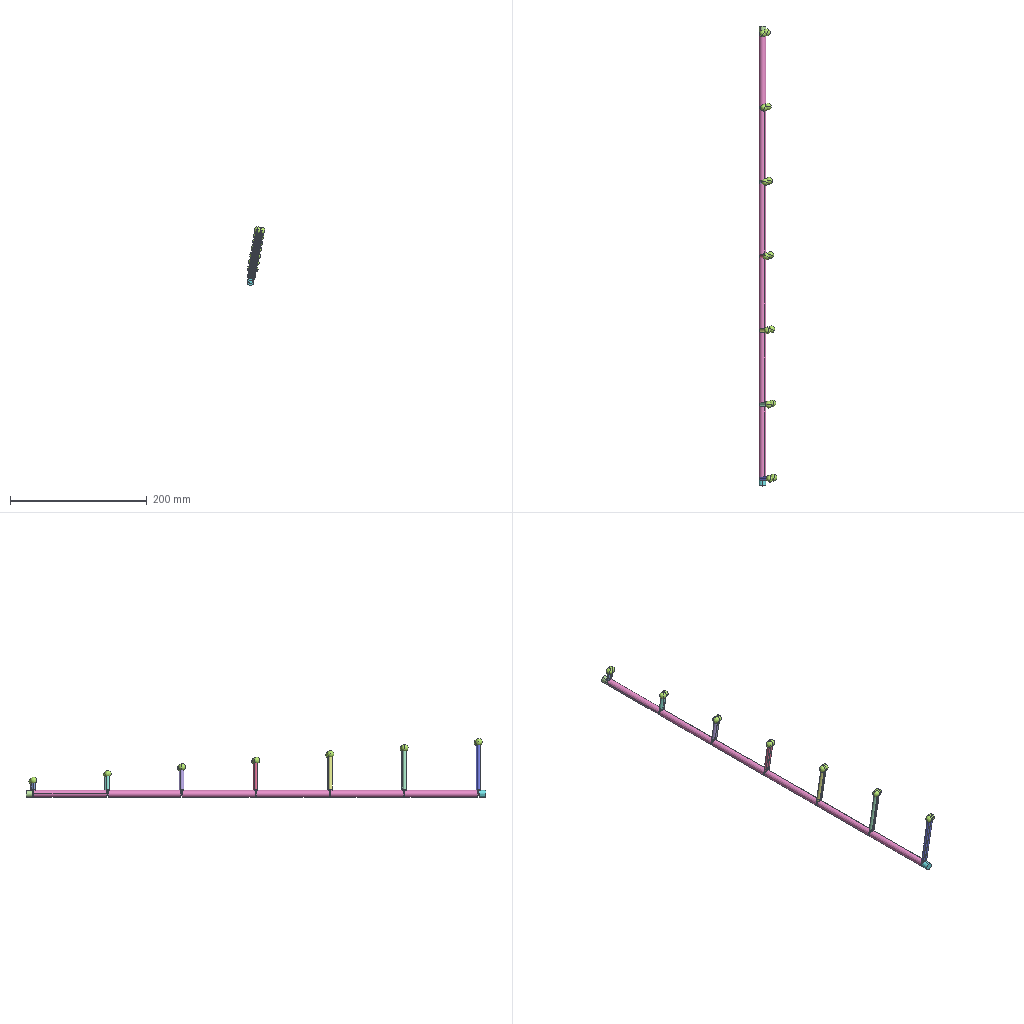Assembly | SolidWorks | 18 different items | 43 placed | box 26 x 673 x 86 mm
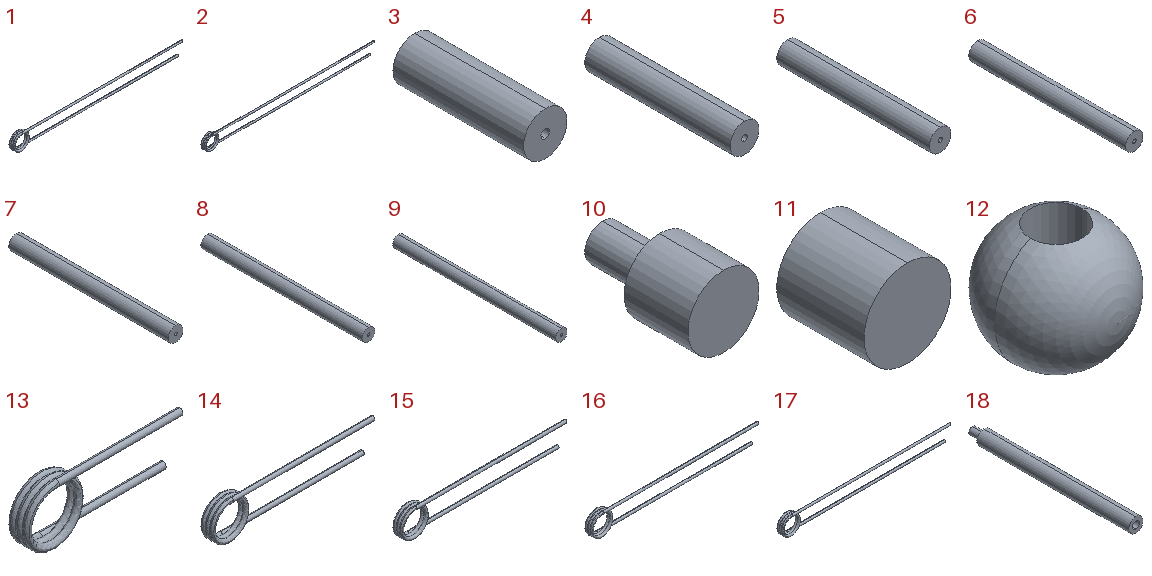Parts list (item | quantity | size | volume | features):
1 | x1 | 64.55 x 2.45 x 6.4 mm | 63.849 mm3 | features MoveFace 2, CompositeCurve 1, Helix 1, Sweep 1
2 | x1 | 73.25 x 2.45 x 6.4 mm | 70.525 mm3 | features MoveFace 2, CompositeCurve 1, Helix 1, Sweep 1
3 | x2 | 5 x 15 x 5 mm | 201.062 mm3 | features Extrusion 1, ICE 1
4 | x2 | 5 x 25 x 5 mm | 326.726 mm3 | features Extrusion 1, ICE 1
5 | x2 | 5 x 35 x 5 mm | 452.389 mm3 | features Extrusion 1, ICE 1
6 | x2 | 5 x 45 x 5 mm | 578.053 mm3 | features Extrusion 1, ICE 1
7 | x2 | 5 x 54.4 x 5 mm | 696.177 mm3 | features Extrusion 1, ICE 1
8 | x2 | 5 x 63.5 x 5 mm | 810.531 mm3 | features Extrusion 1, ICE 1
9 | x2 | 5 x 72.2 x 5 mm | 919.858 mm3 | features Extrusion 1, ICE 1, MoveFace 1
10 | x1 | 10 x 16.95 x 10 mm | 860.011 mm3 | features Extrusion 1, ICE 1
11 | x1 | 10 x 10 x 10 mm | 628.319 mm3 | features Extrusion 1, ICE 1
12 | x14 | 10 x 10 x 9.538 mm | 437.796 mm3 | features HoleWzd 1, Revolution 1
13 | x1 | 16.05 x 2.45 x 6.4 mm | 26.63 mm3 | features CompositeCurve 1, Helix 1, Sweep 1
14 | x1 | 26.05 x 2.45 x 6.4 mm | 34.304 mm3 | features CompositeCurve 1, Helix 1, MoveFace 1, Sweep 1
15 | x1 | 36.05 x 2.45 x 6.4 mm | 41.978 mm3 | features CompositeCurve 1, Helix 1, MoveFace 1, Sweep 1
16 | x1 | 46.05 x 2.45 x 6.4 mm | 49.652 mm3 | features CompositeCurve 1, Helix 1, MoveFace 1, Sweep 1
17 | x1 | 55.45 x 2.45 x 6.4 mm | 56.865 mm3 | features MoveFace 2, CompositeCurve 1, Helix 1, Sweep 1
18 | x6 | 10 x 114.5 x 10 mm | 8325 mm3 | features ICE 2, Extrusion 1
Mates (type | each side: item.copy, entity, surface, feature):
Concentric | 3.1 face cylinder Boss-Extrude1 | 12.1 face cylinder M5 Tapped Hole1
Coincident | 3.1 face plane Boss-Extrude1 | 12.1 edge
Coincident | 12.2 edge | 3.2 face plane Boss-Extrude1
Concentric | 12.2 face sphere Revolve1 | 3.2 face cylinder Boss-Extrude1
Concentric | 13.1 face cylinder Sweep2 | 3.1 face cylinder Boss-Extrude1
Concentric | 13.1 face cylinder Sweep2 | 3.2 face cylinder Boss-Extrude1
Concentric | 14.1 face cylinder Sweep2 | 4.1 face cylinder Boss-Extrude1
Concentric | 14.1 face cylinder Sweep2 | 4.2 face cylinder Boss-Extrude1
Concentric | 12.3 face cylinder M5 Tapped Hole1 | 4.1 face cylinder Boss-Extrude1
Concentric | 12.4 face cylinder M5 Tapped Hole1 | 4.2 face cylinder Boss-Extrude1
Coincident | 12.3 edge | 4.1 face plane Boss-Extrude1
Coincident | 12.4 edge | 4.2 face plane Boss-Extrude1
Coincident | 4.2 face plane Boss-Extrude1 | 4.1 face plane Boss-Extrude1
Parallel | 13.1 face cylinder Sweep2 | 14.1 face cylinder Sweep2
Coincident | 3.1 face plane Boss-Extrude1 | 3.2 face plane Boss-Extrude1
Coincident | 3.1 face plane Boss-Extrude1 | 4.1 face plane Boss-Extrude1
Concentric | 5.1 face cylinder Boss-Extrude1 | 12.5 face cylinder M5 Tapped Hole1
Concentric | 5.2 face cylinder Boss-Extrude1 | 12.6 face cylinder M5 Tapped Hole1
Coincident | 5.1 face plane Boss-Extrude1 | 12.5 edge
Coincident | 5.2 face plane Boss-Extrude1 | 12.6 edge
Concentric | 15.1 face cylinder Sweep2 | 5.2 face cylinder Boss-Extrude1
Concentric | 15.1 face cylinder Sweep2 | 5.1 face cylinder Boss-Extrude1
Coincident | 5.2 face plane Boss-Extrude1 | 5.1 face plane Boss-Extrude1
Coincident | 4.1 face plane Boss-Extrude1 | 5.2 face plane Boss-Extrude1
Concentric | 6.1 face cylinder Boss-Extrude1 | 12.7 face cylinder M5 Tapped Hole1
Concentric | 6.2 face cylinder Boss-Extrude1 | 12.8 face cylinder M5 Tapped Hole1
Coincident | 6.2 face plane Boss-Extrude1 | 12.8 edge
Coincident | 6.1 face plane Boss-Extrude1 | 12.7 edge
Concentric | 16.1 face cylinder Sweep2 | 6.1 face cylinder Boss-Extrude1
Concentric | 16.1 face cylinder Sweep2 | 6.2 face cylinder Boss-Extrude1
Coincident | 5.1 face plane Boss-Extrude1 | 6.2 face plane Boss-Extrude1 | 2 times
Coincident | 6.2 edge | 6.1 face plane Boss-Extrude1
Concentric | 7.1 face cylinder Boss-Extrude1 | 12.9 face cylinder M5 Tapped Hole1
Concentric | 7.2 face cylinder Boss-Extrude1 | 12.10 face cylinder M5 Tapped Hole1
Coincident | 7.1 face plane Boss-Extrude1 | 12.9 edge
Coincident | 7.2 face plane Boss-Extrude1 | 12.10 edge
Concentric | 17.1 face cylinder Sweep2 | 7.2 face cylinder Boss-Extrude1
Concentric | 17.1 face cylinder Sweep2 | 7.1 face cylinder Boss-Extrude1
Coincident | 7.1 face plane Boss-Extrude1 | 7.2 face plane Boss-Extrude1
Parallel | 16.1 face cylinder Sweep2 | 17.1 face cylinder Sweep2
Coincident | 6.1 face plane Boss-Extrude1 | 7.1 face plane Boss-Extrude1
Concentric | 1.1 face cylinder Sweep2 | 8.1 face cylinder Boss-Extrude1
Concentric | 1.1 face cylinder Sweep2 | 8.2 face cylinder Boss-Extrude1
Concentric | 8.2 face cylinder Boss-Extrude1 | 12.11 edge
Concentric | 8.1 face cylinder Boss-Extrude1 | 12.12 face cylinder M5 Tapped Hole1
Coincident | 8.1 face plane Boss-Extrude1 | 12.12 edge
Coincident | 8.2 face plane Boss-Extrude1 | 12.11 edge
Coincident | 8.2 face plane Boss-Extrude1 | 8.1 face plane Boss-Extrude1
Coincident | 7.2 face plane Boss-Extrude1 | 8.1 face plane Boss-Extrude1
Concentric | 9.1 face cylinder Boss-Extrude1 | 12.13 face cylinder M5 Tapped Hole1
Concentric | 9.2 face cylinder Boss-Extrude1 | 12.14 face cylinder M5 Tapped Hole1
Coincident | 9.2 face plane Boss-Extrude1 | 12.14 edge
Coincident | 9.1 face plane Boss-Extrude1 | 12.13 edge
Concentric | 2.1 face cylinder Sweep2 | 9.1 face cylinder Boss-Extrude1
Concentric | 2.1 face cylinder Sweep2 | 9.2 face cylinder Boss-Extrude1
Coincident | 9.2 face plane Boss-Extrude1 | 9.1 face plane Boss-Extrude1
Coincident | 8.2 face plane Boss-Extrude1 | 9.2 face plane Boss-Extrude1
Concentric | 13.1 select_type:24 | 10.1 face cylinder Boss-Extrude1
Tangent | 13.1 face cylinder Sweep2 | 10.1 face plane Boss-Extrude1
Concentric | 10.1 face cylinder Boss-Extrude1 | 18.1 face cylinder Boss-Extrude1
Tangent | 13.1 face cylinder Sweep2 | 18.1 face plane Boss-Extrude1
Concentric | 18.1 face cylinder Boss-Extrude1 | 18.2 face cylinder Boss-Extrude1
Tangent | 14.1 face cylinder Sweep2 | 18.2 face plane Boss-Extrude1
Concentric | 18.2 face cylinder Boss-Extrude2 | 18.3 face cylinder Boss-Extrude1
Tangent | 15.1 face cylinder Sweep2 | 18.3 face plane Boss-Extrude1
Concentric | 18.3 face cylinder Boss-Extrude2 | 18.4 face cylinder Boss-Extrude1
Tangent | 16.1 face cylinder Sweep2 | 18.4 face plane Boss-Extrude1
Concentric | 18.4 face cylinder Boss-Extrude2 | 18.5 face cylinder Boss-Extrude1
Tangent | 17.1 face cylinder Sweep2 | 18.5 face plane Boss-Extrude1
Concentric | 18.5 face cylinder Boss-Extrude2 | 18.6 face cylinder Boss-Extrude1
Tangent | 1.1 face cylinder Sweep2 | 18.6 face plane Boss-Extrude1
Concentric | 18.6 face cylinder Boss-Extrude2 | 11.1 face cylinder Cut-Extrude1
Tangent | 2.1 face cylinder Sweep2 | 11.1 face plane Boss-Extrude1